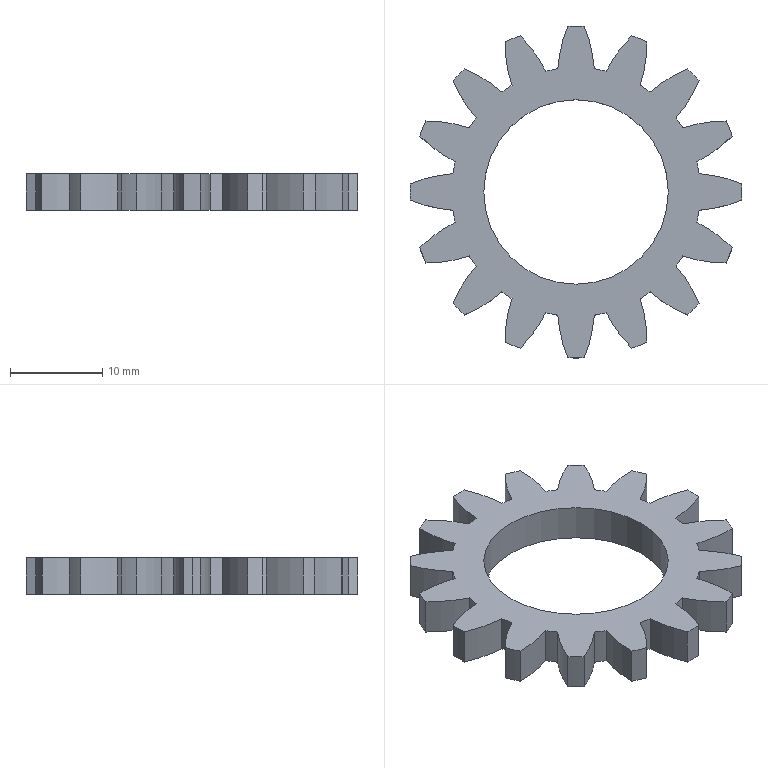Part | SolidWorks | features Extrusion 1 | 1 solid | 71 faces | box 36 x 36 x 4 mm | volume 1937 mm3 | cylinder 69 | plane 2 | commonest cylinder face diameters 29.381 x34 36 x17 27 x16 20 x2